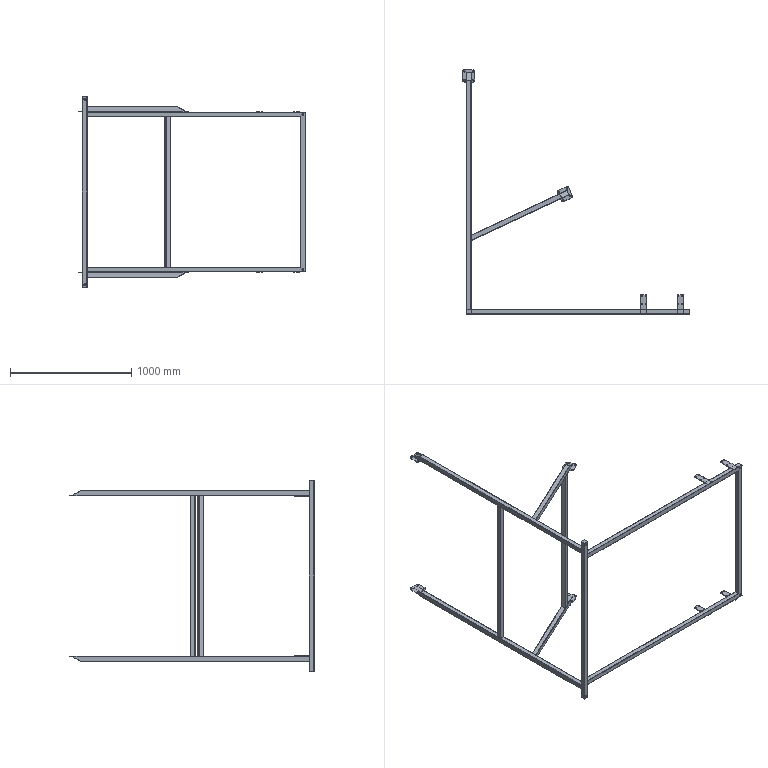Part | STEP file | Produce dryer-Conveyor frame_Default<As Machined> | 19 solids | 420 faces | box 1870 x 2016 x 1574 mm | volume 3631484 mm3 | cylinder 226 | plane 194 | commonest cylinder face diameters 4 x67 1 x41 9 x32 11 x32 16 x20 30 x18